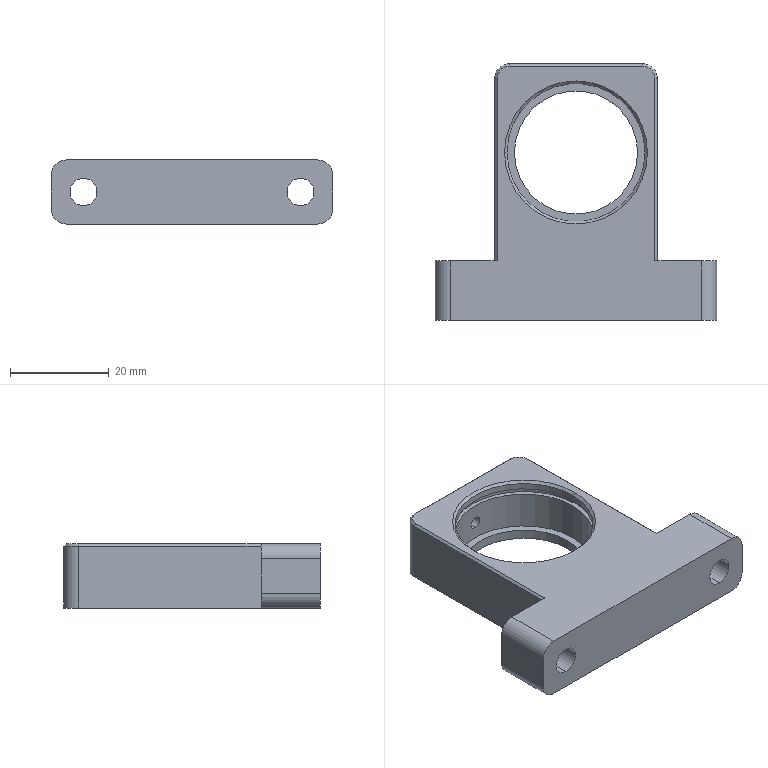Part | NX | features BREP 1 | 1 solid | 62 faces | box 57 x 52 x 13 mm | volume 16656 mm3 | cylinder 32 | plane 18 | cone 12 | commonest cylinder face diameters 2.5 x10 6 x6 5.5 x4 10 x4 28 x4 25 x2